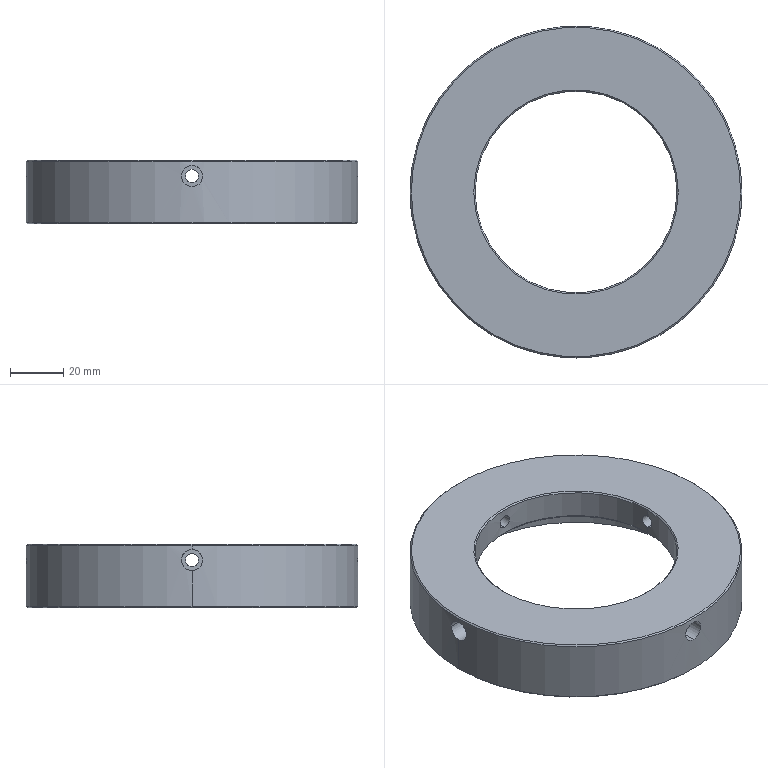Part | STEP file | 2006 Limit side plate B | 1 solid | 53 faces | box 125 x 125 x 24 mm | volume 134168 mm3 | cylinder 30 | cone 16 | plane 7 | commonest cylinder face diameters 3.3 x8 5 x8 8 x8 76 x2 104 x2 125 x2